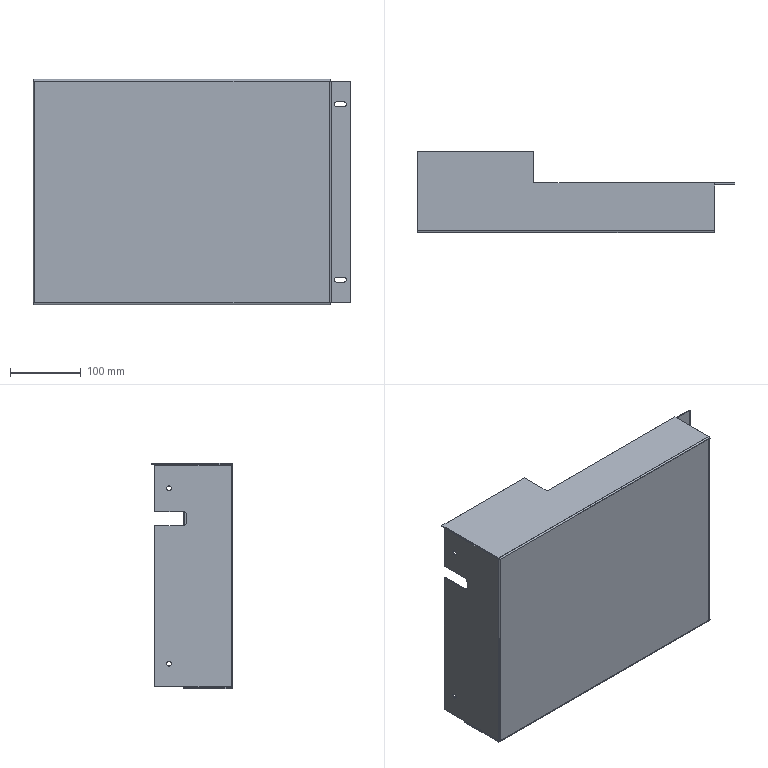Part | STEP file | PN_0030_bent plate_default_machined_ | 1 solid | 58 faces | box 449 x 115 x 318 mm | volume 391309 mm3 | plane 38 | cylinder 20 | commonest cylinder face diameters 1.473 x5 4.473 x5 6.5 x4 7 x4 10 x2